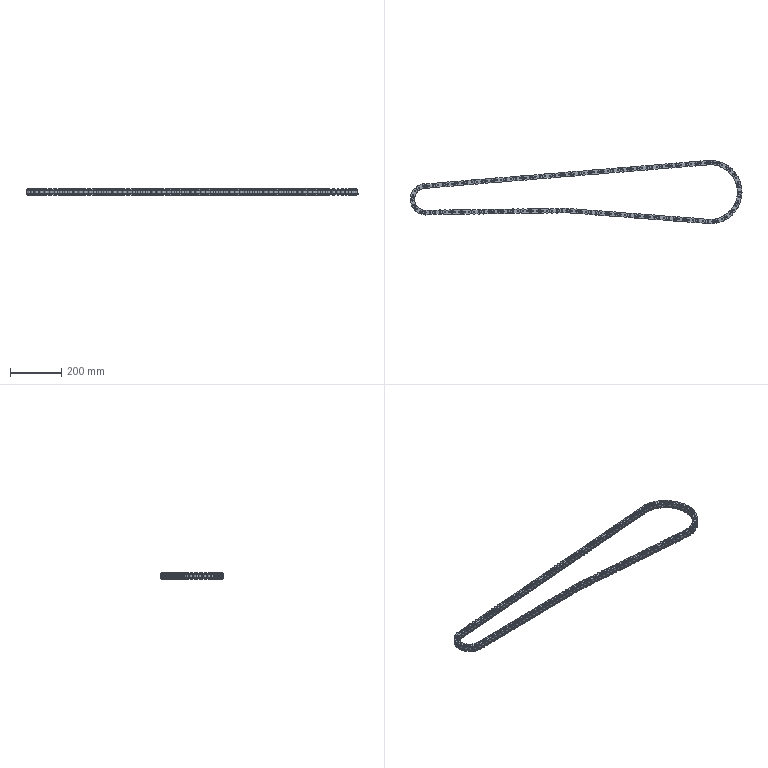Part | SolidWorks | features Boss 3, CurvePattern 2, Chamfer 1, CompositeCurve 1, Extrusion 1, MirrorPattern 1, MirrorSolid 1 | 219 solids | 4380 faces | volume 653125 mm3 | cylinder 2920 | plane 876 | cone 584 | commonest cylinder face diameters 5.96 x1168 18.08 x876 83.184 x584 11.91 x292